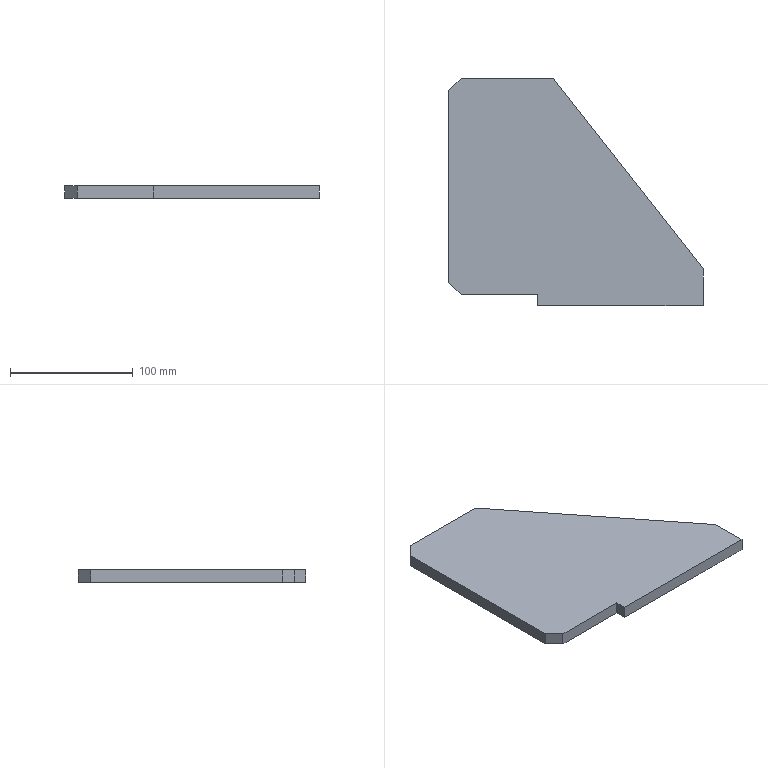Part | STEP file | E3-顶部Beam筋Plate 2 | 1 solid | 11 faces | box 207 x 185 x 10 mm | volume 280920 mm3 | plane 11
STEP:
#1=CARTESIAN_POINT('',(0.,0.,0.));
#2=DIRECTION('',(0.,0.,1.));
#3=DIRECTION('',(1.,0.,0.));
#4=AXIS2_PLACEMENT_3D('',#1,#2,#3);
#5=CARTESIAN_POINT('',(207.,21.,5.));
#6=VERTEX_POINT('',#5);
#7=CARTESIAN_POINT('',(207.,-9.,5.));
#8=VERTEX_POINT('',#7);
#9=CARTESIAN_POINT('',(207.,0.,5.));
#10=DIRECTION('',(0.,-1.,0.));
#11=VECTOR('',#10,1.);
#12=LINE('',#9,#11);
#13=CARTESIAN_POINT('',(207.,0.,-5.));
#14=DIRECTION('',(1.,0.,0.));
#15=DIRECTION('',(0.,0.,1.));
#16=AXIS2_PLACEMENT_3D('',#13,#14,#15);
#17=PLANE('',#16);
#18=CARTESIAN_POINT('',(10.,0.));
#19=DIRECTION('',(0.,1.));
#20=VECTOR('',#19,1.);
#21=LINE('',#18,#20);
#22=(GEOMETRIC_REPRESENTATION_CONTEXT(2)PARAMETRIC_REPRESENTATION_CONTEXT()REPRESENTATION_CONTEXT('',''));
#23=DEFINITIONAL_REPRESENTATION('',(#21),#22);
#24=PCURVE('',#17,#23);
#25=CARTESIAN_POINT('',(0.,0.,5.));
#26=DIRECTION('',(0.,0.,-1.));
#27=DIRECTION('',(1.,0.,0.));
#28=AXIS2_PLACEMENT_3D('',#25,#26,#27);
#29=PLANE('',#28);
#30=CARTESIAN_POINT('',(207.,0.));
#31=DIRECTION('',(0.,1.));
#32=VECTOR('',#31,1.);
#33=LINE('',#30,#32);
#34=(GEOMETRIC_REPRESENTATION_CONTEXT(2)PARAMETRIC_REPRESENTATION_CONTEXT()REPRESENTATION_CONTEXT('',''));
#35=DEFINITIONAL_REPRESENTATION('',(#33),#34);
#36=PCURVE('',#29,#35);
#37=SURFACE_CURVE('',#12,(#24,#36),.PCURVE_S1.);
#38=EDGE_CURVE('',#6,#8,#37,.T.);
#39=ORIENTED_EDGE('',*,*,#38,.T.);
#40=CARTESIAN_POINT('',(207.,-9.,-5.));
#41=VERTEX_POINT('',#40);
#42=CARTESIAN_POINT('',(207.,-9.,-5.));
#43=DIRECTION('',(0.,0.,1.));
#44=VECTOR('',#43,1.);
#45=LINE('',#42,#44);
#46=CARTESIAN_POINT('',(0.,9.));
#47=DIRECTION('',(1.,0.));
#48=VECTOR('',#47,1.);
#49=LINE('',#46,#48);
#50=(GEOMETRIC_REPRESENTATION_CONTEXT(2)PARAMETRIC_REPRESENTATION_CONTEXT()REPRESENTATION_CONTEXT('',''));
#51=DEFINITIONAL_REPRESENTATION('',(#49),#50);
#52=PCURVE('',#17,#51);
#53=CARTESIAN_POINT('',(0.,-9.,-5.));
#54=DIRECTION('',(0.,1.,0.));
#55=DIRECTION('',(-1.,0.,0.));
#56=AXIS2_PLACEMENT_3D('',#53,#54,#55);
#57=PLANE('',#56);
#58=CARTESIAN_POINT('',(-207.,0.));
#59=DIRECTION('',(0.,1.));
#60=VECTOR('',#59,1.);
#61=LINE('',#58,#60);
#62=(GEOMETRIC_REPRESENTATION_CONTEXT(2)PARAMETRIC_REPRESENTATION_CONTEXT()REPRESENTATION_CONTEXT('',''));
#63=DEFINITIONAL_REPRESENTATION('',(#61),#62);
#64=PCURVE('',#57,#63);
#65=SURFACE_CURVE('',#45,(#52,#64),.PCURVE_S1.);
#66=EDGE_CURVE('',#41,#8,#65,.T.);
#67=ORIENTED_EDGE('',*,*,#66,.F.);
#68=CARTESIAN_POINT('',(207.,21.,-5.));
#69=VERTEX_POINT('',#68);
#70=CARTESIAN_POINT('',(207.,0.,-5.));
#71=DIRECTION('',(0.,-1.,0.));
#72=VECTOR('',#71,1.);
#73=LINE('',#70,#72);
#74=CARTESIAN_POINT('',(0.,0.));
#75=DIRECTION('',(0.,1.));
#76=VECTOR('',#75,1.);
#77=LINE('',#74,#76);
#78=(GEOMETRIC_REPRESENTATION_CONTEXT(2)PARAMETRIC_REPRESENTATION_CONTEXT()REPRESENTATION_CONTEXT('',''));
#79=DEFINITIONAL_REPRESENTATION('',(#77),#78);
#80=PCURVE('',#17,#79);
#81=CARTESIAN_POINT('',(0.,0.,-5.));
#82=DIRECTION('',(0.,0.,-1.));
#83=DIRECTION('',(1.,0.,0.));
#84=AXIS2_PLACEMENT_3D('',#81,#82,#83);
#85=PLANE('',#84);
#86=CARTESIAN_POINT('',(207.,0.));
#87=DIRECTION('',(0.,1.));
#88=VECTOR('',#87,1.);
#89=LINE('',#86,#88);
#90=(GEOMETRIC_REPRESENTATION_CONTEXT(2)PARAMETRIC_REPRESENTATION_CONTEXT()REPRESENTATION_CONTEXT('',''));
#91=DEFINITIONAL_REPRESENTATION('',(#89),#90);
#92=PCURVE('',#85,#91);
#93=SURFACE_CURVE('',#73,(#80,#92),.PCURVE_S1.);
#94=EDGE_CURVE('',#69,#41,#93,.T.);
#95=ORIENTED_EDGE('',*,*,#94,.F.);
#96=CARTESIAN_POINT('',(207.,21.,-5.));
#97=DIRECTION('',(0.,0.,1.));
#98=VECTOR('',#97,1.);
#99=LINE('',#96,#98);
#100=CARTESIAN_POINT('',(0.,-21.));
#101=DIRECTION('',(1.,0.));
#102=VECTOR('',#101,1.);
#103=LINE('',#100,#102);
#104=(GEOMETRIC_REPRESENTATION_CONTEXT(2)PARAMETRIC_REPRESENTATION_CONTEXT()REPRESENTATION_CONTEXT('',''));
#105=DEFINITIONAL_REPRESENTATION('',(#103),#104);
#106=PCURVE('',#17,#105);
#107=CARTESIAN_POINT('',(138.022,108.636,-5.));
#108=DIRECTION('',(0.7858,0.6185,0.));
#109=DIRECTION('',(-0.6185,0.7858,0.));
#110=AXIS2_PLACEMENT_3D('',#107,#108,#109);
#111=PLANE('',#110);
#112=CARTESIAN_POINT('',(-111.526,0.));
#113=DIRECTION('',(0.,1.));
#114=VECTOR('',#113,1.);
#115=LINE('',#112,#114);
#116=(GEOMETRIC_REPRESENTATION_CONTEXT(2)PARAMETRIC_REPRESENTATION_CONTEXT()REPRESENTATION_CONTEXT('',''));
#117=DEFINITIONAL_REPRESENTATION('',(#115),#116);
#118=PCURVE('',#111,#117);
#119=SURFACE_CURVE('',#99,(#106,#118),.PCURVE_S1.);
#120=EDGE_CURVE('',#69,#6,#119,.T.);
#121=ORIENTED_EDGE('',*,*,#120,.T.);
#122=EDGE_LOOP('',(#39,#67,#95,#121));
#123=FACE_BOUND('',#122,.T.);
#124=ADVANCED_FACE('',(#123),#17,.T.);
#125=CARTESIAN_POINT('',(85.,176.,5.));
#126=VERTEX_POINT('',#125);
#127=CARTESIAN_POINT('',(138.022,108.636,5.));
#128=DIRECTION('',(0.6185,-0.7858,0.));
#129=VECTOR('',#128,1.);
#130=LINE('',#127,#129);
#131=CARTESIAN_POINT('',(0.,10.));
#132=DIRECTION('',(-1.,0.));
#133=VECTOR('',#132,1.);
#134=LINE('',#131,#133);
#135=(GEOMETRIC_REPRESENTATION_CONTEXT(2)PARAMETRIC_REPRESENTATION_CONTEXT()REPRESENTATION_CONTEXT('',''));
#136=DEFINITIONAL_REPRESENTATION('',(#134),#135);
#137=PCURVE('',#111,#136);
#138=CARTESIAN_POINT('',(138.022,-108.636));
#139=DIRECTION('',(0.6185,0.7858));
#140=VECTOR('',#139,1.);
#141=LINE('',#138,#140);
#142=(GEOMETRIC_REPRESENTATION_CONTEXT(2)PARAMETRIC_REPRESENTATION_CONTEXT()REPRESENTATION_CONTEXT('',''));
#143=DEFINITIONAL_REPRESENTATION('',(#141),#142);
#144=PCURVE('',#29,#143);
#145=SURFACE_CURVE('',#130,(#137,#144),.PCURVE_S1.);
#146=EDGE_CURVE('',#126,#6,#145,.T.);
#147=ORIENTED_EDGE('',*,*,#146,.T.);
#148=ORIENTED_EDGE('',*,*,#120,.F.);
#149=CARTESIAN_POINT('',(85.,176.,-5.));
#150=VERTEX_POINT('',#149);
#151=CARTESIAN_POINT('',(138.022,108.636,-5.));
#152=DIRECTION('',(0.6185,-0.7858,0.));
#153=VECTOR('',#152,1.);
#154=LINE('',#151,#153);
#155=CARTESIAN_POINT('',(0.,0.));
#156=DIRECTION('',(-1.,0.));
#157=VECTOR('',#156,1.);
#158=LINE('',#155,#157);
#159=(GEOMETRIC_REPRESENTATION_CONTEXT(2)PARAMETRIC_REPRESENTATION_CONTEXT()REPRESENTATION_CONTEXT('',''));
#160=DEFINITIONAL_REPRESENTATION('',(#158),#159);
#161=PCURVE('',#111,#160);
#162=CARTESIAN_POINT('',(138.022,-108.636));
#163=DIRECTION('',(0.6185,0.7858));
#164=VECTOR('',#163,1.);
#165=LINE('',#162,#164);
#166=(GEOMETRIC_REPRESENTATION_CONTEXT(2)PARAMETRIC_REPRESENTATION_CONTEXT()REPRESENTATION_CONTEXT('',''));
#167=DEFINITIONAL_REPRESENTATION('',(#165),#166);
#168=PCURVE('',#85,#167);
#169=SURFACE_CURVE('',#154,(#161,#168),.PCURVE_S1.);
#170=EDGE_CURVE('',#150,#69,#169,.T.);
#171=ORIENTED_EDGE('',*,*,#170,.F.);
#172=CARTESIAN_POINT('',(85.,176.,-5.));
#173=DIRECTION('',(0.,0.,1.));
#174=VECTOR('',#173,1.);
#175=LINE('',#172,#174);
#176=CARTESIAN_POINT('',(85.727,0.));
#177=DIRECTION('',(0.,1.));
#178=VECTOR('',#177,1.);
#179=LINE('',#176,#178);
#180=(GEOMETRIC_REPRESENTATION_CONTEXT(2)PARAMETRIC_REPRESENTATION_CONTEXT()REPRESENTATION_CONTEXT('',''));
#181=DEFINITIONAL_REPRESENTATION('',(#179),#180);
#182=PCURVE('',#111,#181);
#183=CARTESIAN_POINT('',(0.,176.,-5.));
#184=DIRECTION('',(0.,1.,0.));
#185=DIRECTION('',(0.,0.,-1.));
#186=AXIS2_PLACEMENT_3D('',#183,#184,#185);
#187=PLANE('',#186);
#188=CARTESIAN_POINT('',(0.,-85.));
#189=DIRECTION('',(-1.,0.));
#190=VECTOR('',#189,1.);
#191=LINE('',#188,#190);
#192=(GEOMETRIC_REPRESENTATION_CONTEXT(2)PARAMETRIC_REPRESENTATION_CONTEXT()REPRESENTATION_CONTEXT('',''));
#193=DEFINITIONAL_REPRESENTATION('',(#191),#192);
#194=PCURVE('',#187,#193);
#195=SURFACE_CURVE('',#175,(#182,#194),.PCURVE_S1.);
#196=EDGE_CURVE('',#150,#126,#195,.T.);
#197=ORIENTED_EDGE('',*,*,#196,.T.);
#198=EDGE_LOOP('',(#147,#148,#171,#197));
#199=FACE_BOUND('',#198,.T.);
#200=ADVANCED_FACE('',(#199),#111,.T.);
#201=CARTESIAN_POINT('',(10.,176.,5.));
#202=VERTEX_POINT('',#201);
#203=CARTESIAN_POINT('',(0.,176.,5.));
#204=DIRECTION('',(1.,0.,0.));
#205=VECTOR('',#204,1.);
#206=LINE('',#203,#205);
#207=CARTESIAN_POINT('',(-10.,0.));
#208=DIRECTION('',(0.,-1.));
#209=VECTOR('',#208,1.);
#210=LINE('',#207,#209);
#211=(GEOMETRIC_REPRESENTATION_CONTEXT(2)PARAMETRIC_REPRESENTATION_CONTEXT()REPRESENTATION_CONTEXT('',''));
#212=DEFINITIONAL_REPRESENTATION('',(#210),#211);
#213=PCURVE('',#187,#212);
#214=CARTESIAN_POINT('',(0.,-176.));
#215=DIRECTION('',(1.,0.));
#216=VECTOR('',#215,1.);
#217=LINE('',#214,#216);
#218=(GEOMETRIC_REPRESENTATION_CONTEXT(2)PARAMETRIC_REPRESENTATION_CONTEXT()REPRESENTATION_CONTEXT('',''));
#219=DEFINITIONAL_REPRESENTATION('',(#217),#218);
#220=PCURVE('',#29,#219);
#221=SURFACE_CURVE('',#206,(#213,#220),.PCURVE_S1.);
#222=EDGE_CURVE('',#202,#126,#221,.T.);
#223=ORIENTED_EDGE('',*,*,#222,.T.);
#224=ORIENTED_EDGE('',*,*,#196,.F.);
#225=CARTESIAN_POINT('',(10.,176.,-5.));
#226=VERTEX_POINT('',#225);
#227=CARTESIAN_POINT('',(0.,176.,-5.));
#228=DIRECTION('',(1.,0.,0.));
#229=VECTOR('',#228,1.);
#230=LINE('',#227,#229);
#231=CARTESIAN_POINT('',(0.,0.));
#232=DIRECTION('',(0.,-1.));
#233=VECTOR('',#232,1.);
#234=LINE('',#231,#233);
#235=(GEOMETRIC_REPRESENTATION_CONTEXT(2)PARAMETRIC_REPRESENTATION_CONTEXT()REPRESENTATION_CONTEXT('',''));
#236=DEFINITIONAL_REPRESENTATION('',(#234),#235);
#237=PCURVE('',#187,#236);
#238=CARTESIAN_POINT('',(0.,-176.));
#239=DIRECTION('',(1.,0.));
#240=VECTOR('',#239,1.);
#241=LINE('',#238,#240);
#242=(GEOMETRIC_REPRESENTATION_CONTEXT(2)PARAMETRIC_REPRESENTATION_CONTEXT()REPRESENTATION_CONTEXT('',''));
#243=DEFINITIONAL_REPRESENTATION('',(#241),#242);
#244=PCURVE('',#85,#243);
#245=SURFACE_CURVE('',#230,(#237,#244),.PCURVE_S1.);
#246=EDGE_CURVE('',#226,#150,#245,.T.);
#247=ORIENTED_EDGE('',*,*,#246,.F.);
#248=CARTESIAN_POINT('',(10.,176.,-5.));
#249=DIRECTION('',(0.,0.,-1.));
#250=VECTOR('',#249,1.);
#251=LINE('',#248,#250);
#252=CARTESIAN_POINT('',(0.,-10.));
#253=DIRECTION('',(1.,0.));
#254=VECTOR('',#253,1.);
#255=LINE('',#252,#254);
#256=(GEOMETRIC_REPRESENTATION_CONTEXT(2)PARAMETRIC_REPRESENTATION_CONTEXT()REPRESENTATION_CONTEXT('',''));
#257=DEFINITIONAL_REPRESENTATION('',(#255),#256);
#258=PCURVE('',#187,#257);
#259=CARTESIAN_POINT('',(0.,166.,-5.));
#260=DIRECTION('',(0.7071,-0.7071,0.));
#261=DIRECTION('',(0.,0.,1.));
#262=AXIS2_PLACEMENT_3D('',#259,#260,#261);
#263=PLANE('',#262);
#264=CARTESIAN_POINT('',(0.,-14.142));
#265=DIRECTION('',(-1.,0.));
#266=VECTOR('',#265,1.);
#267=LINE('',#264,#266);
#268=(GEOMETRIC_REPRESENTATION_CONTEXT(2)PARAMETRIC_REPRESENTATION_CONTEXT()REPRESENTATION_CONTEXT('',''));
#269=DEFINITIONAL_REPRESENTATION('',(#267),#268);
#270=PCURVE('',#263,#269);
#271=SURFACE_CURVE('',#251,(#258,#270),.PCURVE_S1.);
#272=EDGE_CURVE('',#202,#226,#271,.T.);
#273=ORIENTED_EDGE('',*,*,#272,.F.);
#274=EDGE_LOOP('',(#223,#224,#247,#273));
#275=FACE_BOUND('',#274,.T.);
#276=ADVANCED_FACE('',(#275),#187,.T.);
#277=CARTESIAN_POINT('',(0.,10.,5.));
#278=VERTEX_POINT('',#277);
#279=CARTESIAN_POINT('',(0.,166.,5.));
#280=VERTEX_POINT('',#279);
#281=CARTESIAN_POINT('',(0.,0.,5.));
#282=DIRECTION('',(0.,1.,0.));
#283=VECTOR('',#282,1.);
#284=LINE('',#281,#283);
#285=CARTESIAN_POINT('',(0.,0.,-5.));
#286=DIRECTION('',(-1.,0.,0.));
#287=DIRECTION('',(0.,0.,-1.));
#288=AXIS2_PLACEMENT_3D('',#285,#286,#287);
#289=PLANE('',#288);
#290=CARTESIAN_POINT('',(-10.,0.));
#291=DIRECTION('',(0.,-1.));
#292=VECTOR('',#291,1.);
#293=LINE('',#290,#292);
#294=(GEOMETRIC_REPRESENTATION_CONTEXT(2)PARAMETRIC_REPRESENTATION_CONTEXT()REPRESENTATION_CONTEXT('',''));
#295=DEFINITIONAL_REPRESENTATION('',(#293),#294);
#296=PCURVE('',#289,#295);
#297=CARTESIAN_POINT('',(0.,0.));
#298=DIRECTION('',(0.,-1.));
#299=VECTOR('',#298,1.);
#300=LINE('',#297,#299);
#301=(GEOMETRIC_REPRESENTATION_CONTEXT(2)PARAMETRIC_REPRESENTATION_CONTEXT()REPRESENTATION_CONTEXT('',''));
#302=DEFINITIONAL_REPRESENTATION('',(#300),#301);
#303=PCURVE('',#29,#302);
#304=SURFACE_CURVE('',#284,(#296,#303),.PCURVE_S1.);
#305=EDGE_CURVE('',#278,#280,#304,.T.);
#306=ORIENTED_EDGE('',*,*,#305,.T.);
#307=CARTESIAN_POINT('',(0.,166.,-5.));
#308=VERTEX_POINT('',#307);
#309=CARTESIAN_POINT('',(0.,166.,-5.));
#310=DIRECTION('',(0.,0.,1.));
#311=VECTOR('',#310,1.);
#312=LINE('',#309,#311);
#313=CARTESIAN_POINT('',(0.,-166.));
#314=DIRECTION('',(-1.,0.));
#315=VECTOR('',#314,1.);
#316=LINE('',#313,#315);
#317=(GEOMETRIC_REPRESENTATION_CONTEXT(2)PARAMETRIC_REPRESENTATION_CONTEXT()REPRESENTATION_CONTEXT('',''));
#318=DEFINITIONAL_REPRESENTATION('',(#316),#317);
#319=PCURVE('',#289,#318);
#320=CARTESIAN_POINT('',(0.,0.));
#321=DIRECTION('',(1.,0.));
#322=VECTOR('',#321,1.);
#323=LINE('',#320,#322);
#324=(GEOMETRIC_REPRESENTATION_CONTEXT(2)PARAMETRIC_REPRESENTATION_CONTEXT()REPRESENTATION_CONTEXT('',''));
#325=DEFINITIONAL_REPRESENTATION('',(#323),#324);
#326=PCURVE('',#263,#325);
#327=SURFACE_CURVE('',#312,(#319,#326),.PCURVE_S1.);
#328=EDGE_CURVE('',#308,#280,#327,.T.);
#329=ORIENTED_EDGE('',*,*,#328,.F.);
#330=CARTESIAN_POINT('',(0.,10.,-5.));
#331=VERTEX_POINT('',#330);
#332=CARTESIAN_POINT('',(0.,0.,-5.));
#333=DIRECTION('',(0.,1.,0.));
#334=VECTOR('',#333,1.);
#335=LINE('',#332,#334);
#336=CARTESIAN_POINT('',(0.,0.));
#337=DIRECTION('',(0.,-1.));
#338=VECTOR('',#337,1.);
#339=LINE('',#336,#338);
#340=(GEOMETRIC_REPRESENTATION_CONTEXT(2)PARAMETRIC_REPRESENTATION_CONTEXT()REPRESENTATION_CONTEXT('',''));
#341=DEFINITIONAL_REPRESENTATION('',(#339),#340);
#342=PCURVE('',#289,#341);
#343=CARTESIAN_POINT('',(0.,0.));
#344=DIRECTION('',(0.,-1.));
#345=VECTOR('',#344,1.);
#346=LINE('',#343,#345);
#347=(GEOMETRIC_REPRESENTATION_CONTEXT(2)PARAMETRIC_REPRESENTATION_CONTEXT()REPRESENTATION_CONTEXT('',''));
#348=DEFINITIONAL_REPRESENTATION('',(#346),#347);
#349=PCURVE('',#85,#348);
#350=SURFACE_CURVE('',#335,(#342,#349),.PCURVE_S1.);
#351=EDGE_CURVE('',#331,#308,#350,.T.);
#352=ORIENTED_EDGE('',*,*,#351,.F.);
#353=CARTESIAN_POINT('',(0.,10.,-5.));
#354=DIRECTION('',(0.,0.,-1.));
#355=VECTOR('',#354,1.);
#356=LINE('',#353,#355);
#357=CARTESIAN_POINT('',(0.,-10.));
#358=DIRECTION('',(1.,0.));
#359=VECTOR('',#358,1.);
#360=LINE('',#357,#359);
#361=(GEOMETRIC_REPRESENTATION_CONTEXT(2)PARAMETRIC_REPRESENTATION_CONTEXT()REPRESENTATION_CONTEXT('',''));
#362=DEFINITIONAL_REPRESENTATION('',(#360),#361);
#363=PCURVE('',#289,#362);
#364=CARTESIAN_POINT('',(10.,0.,-5.));
#365=DIRECTION('',(-0.7071,-0.7071,0.));
#366=DIRECTION('',(0.,0.,-1.));
#367=AXIS2_PLACEMENT_3D('',#364,#365,#366);
#368=PLANE('',#367);
#369=CARTESIAN_POINT('',(0.,-14.142));
#370=DIRECTION('',(1.,0.));
#371=VECTOR('',#370,1.);
#372=LINE('',#369,#371);
#373=(GEOMETRIC_REPRESENTATION_CONTEXT(2)PARAMETRIC_REPRESENTATION_CONTEXT()REPRESENTATION_CONTEXT('',''));
#374=DEFINITIONAL_REPRESENTATION('',(#372),#373);
#375=PCURVE('',#368,#374);
#376=SURFACE_CURVE('',#356,(#363,#375),.PCURVE_S1.);
#377=EDGE_CURVE('',#278,#331,#376,.T.);
#378=ORIENTED_EDGE('',*,*,#377,.F.);
#379=EDGE_LOOP('',(#306,#329,#352,#378));
#380=FACE_BOUND('',#379,.T.);
#381=ADVANCED_FACE('',(#380),#289,.T.);
#382=CARTESIAN_POINT('',(10.,0.,-5.));
#383=VERTEX_POINT('',#382);
#384=CARTESIAN_POINT('',(72.,0.,-5.));
#385=VERTEX_POINT('',#384);
#386=CARTESIAN_POINT('',(0.,0.,-5.));
#387=DIRECTION('',(1.,0.,0.));
#388=VECTOR('',#387,1.);
#389=LINE('',#386,#388);
#390=CARTESIAN_POINT('',(0.,0.,-5.));
#391=DIRECTION('',(0.,1.,0.));
#392=DIRECTION('',(0.,0.,-1.));
#393=AXIS2_PLACEMENT_3D('',#390,#391,#392);
#394=PLANE('',#393);
#395=CARTESIAN_POINT('',(0.,0.));
#396=DIRECTION('',(0.,-1.));
#397=VECTOR('',#396,1.);
#398=LINE('',#395,#397);
#399=(GEOMETRIC_REPRESENTATION_CONTEXT(2)PARAMETRIC_REPRESENTATION_CONTEXT()REPRESENTATION_CONTEXT('',''));
#400=DEFINITIONAL_REPRESENTATION('',(#398),#399);
#401=PCURVE('',#394,#400);
#402=CARTESIAN_POINT('',(0.,0.));
#403=DIRECTION('',(1.,0.));
#404=VECTOR('',#403,1.);
#405=LINE('',#402,#404);
#406=(GEOMETRIC_REPRESENTATION_CONTEXT(2)PARAMETRIC_REPRESENTATION_CONTEXT()REPRESENTATION_CONTEXT('',''));
#407=DEFINITIONAL_REPRESENTATION('',(#405),#406);
#408=PCURVE('',#85,#407);
#409=SURFACE_CURVE('',#389,(#401,#408),.PCURVE_S1.);
#410=EDGE_CURVE('',#383,#385,#409,.T.);
#411=ORIENTED_EDGE('',*,*,#410,.T.);
#412=CARTESIAN_POINT('',(72.,0.,5.));
#413=VERTEX_POINT('',#412);
#414=CARTESIAN_POINT('',(72.,0.,-5.));
#415=DIRECTION('',(0.,0.,1.));
#416=VECTOR('',#415,1.);
#417=LINE('',#414,#416);
#418=CARTESIAN_POINT('',(0.,-72.));
#419=DIRECTION('',(-1.,0.));
#420=VECTOR('',#419,1.);
#421=LINE('',#418,#420);
#422=(GEOMETRIC_REPRESENTATION_CONTEXT(2)PARAMETRIC_REPRESENTATION_CONTEXT()REPRESENTATION_CONTEXT('',''));
#423=DEFINITIONAL_REPRESENTATION('',(#421),#422);
#424=PCURVE('',#394,#423);
#425=CARTESIAN_POINT('',(72.,0.,-5.));
#426=DIRECTION('',(1.,0.,0.));
#427=DIRECTION('',(0.,0.,1.));
#428=AXIS2_PLACEMENT_3D('',#425,#426,#427);
#429=PLANE('',#428);
#430=CARTESIAN_POINT('',(0.,0.));
#431=DIRECTION('',(1.,0.));
#432=VECTOR('',#431,1.);
#433=LINE('',#430,#432);
#434=(GEOMETRIC_REPRESENTATION_CONTEXT(2)PARAMETRIC_REPRESENTATION_CONTEXT()REPRESENTATION_CONTEXT('',''));
#435=DEFINITIONAL_REPRESENTATION('',(#433),#434);
#436=PCURVE('',#429,#435);
#437=SURFACE_CURVE('',#417,(#424,#436),.PCURVE_S1.);
#438=EDGE_CURVE('',#385,#413,#437,.T.);
#439=ORIENTED_EDGE('',*,*,#438,.T.);
#440=CARTESIAN_POINT('',(10.,0.,5.));
#441=VERTEX_POINT('',#440);
#442=CARTESIAN_POINT('',(0.,0.,5.));
#443=DIRECTION('',(1.,0.,0.));
#444=VECTOR('',#443,1.);
#445=LINE('',#442,#444);
#446=CARTESIAN_POINT('',(-10.,0.));
#447=DIRECTION('',(0.,-1.));
#448=VECTOR('',#447,1.);
#449=LINE('',#446,#448);
#450=(GEOMETRIC_REPRESENTATION_CONTEXT(2)PARAMETRIC_REPRESENTATION_CONTEXT()REPRESENTATION_CONTEXT('',''));
#451=DEFINITIONAL_REPRESENTATION('',(#449),#450);
#452=PCURVE('',#394,#451);
#453=CARTESIAN_POINT('',(0.,0.));
#454=DIRECTION('',(1.,0.));
#455=VECTOR('',#454,1.);
#456=LINE('',#453,#455);
#457=(GEOMETRIC_REPRESENTATION_CONTEXT(2)PARAMETRIC_REPRESENTATION_CONTEXT()REPRESENTATION_CONTEXT('',''));
#458=DEFINITIONAL_REPRESENTATION('',(#456),#457);
#459=PCURVE('',#29,#458);
#460=SURFACE_CURVE('',#445,(#452,#459),.PCURVE_S1.);
#461=EDGE_CURVE('',#441,#413,#460,.T.);
#462=ORIENTED_EDGE('',*,*,#461,.F.);
#463=CARTESIAN_POINT('',(10.,0.,5.));
#464=DIRECTION('',(0.,0.,1.));
#465=VECTOR('',#464,1.);
#466=LINE('',#463,#465);
#467=CARTESIAN_POINT('',(-10.,-10.));
#468=DIRECTION('',(-1.,0.));
#469=VECTOR('',#468,1.);
#470=LINE('',#467,#469);
#471=(GEOMETRIC_REPRESENTATION_CONTEXT(2)PARAMETRIC_REPRESENTATION_CONTEXT()REPRESENTATION_CONTEXT('',''));
#472=DEFINITIONAL_REPRESENTATION('',(#470),#471);
#473=PCURVE('',#394,#472);
#474=CARTESIAN_POINT('',(-10.,0.));
#475=DIRECTION('',(-1.,0.));
#476=VECTOR('',#475,1.);
#477=LINE('',#474,#476);
#478=(GEOMETRIC_REPRESENTATION_CONTEXT(2)PARAMETRIC_REPRESENTATION_CONTEXT()REPRESENTATION_CONTEXT('',''));
#479=DEFINITIONAL_REPRESENTATION('',(#477),#478);
#480=PCURVE('',#368,#479);
#481=SURFACE_CURVE('',#466,(#473,#480),.PCURVE_S1.);
#482=EDGE_CURVE('',#383,#441,#481,.T.);
#483=ORIENTED_EDGE('',*,*,#482,.F.);
#484=EDGE_LOOP('',(#411,#439,#462,#483));
#485=FACE_BOUND('',#484,.T.);
#486=ADVANCED_FACE('',(#485),#394,.F.);
#487=CARTESIAN_POINT('',(72.,-9.,5.));
#488=VERTEX_POINT('',#487);
#489=CARTESIAN_POINT('',(72.,0.,5.));
#490=DIRECTION('',(0.,-1.,0.));
#491=VECTOR('',#490,1.);
#492=LINE('',#489,#491);
#493=CARTESIAN_POINT('',(10.,0.));
#494=DIRECTION('',(0.,1.));
#495=VECTOR('',#494,1.);
#496=LINE('',#493,#495);
#497=(GEOMETRIC_REPRESENTATION_CONTEXT(2)PARAMETRIC_REPRESENTATION_CONTEXT()REPRESENTATION_CONTEXT('',''));
#498=DEFINITIONAL_REPRESENTATION('',(#496),#497);
#499=PCURVE('',#429,#498);
#500=CARTESIAN_POINT('',(72.,0.));
#501=DIRECTION('',(0.,1.));
#502=VECTOR('',#501,1.);
#503=LINE('',#500,#502);
#504=(GEOMETRIC_REPRESENTATION_CONTEXT(2)PARAMETRIC_REPRESENTATION_CONTEXT()REPRESENTATION_CONTEXT('',''));
#505=DEFINITIONAL_REPRESENTATION('',(#503),#504);
#506=PCURVE('',#29,#505);
#507=SURFACE_CURVE('',#492,(#499,#506),.PCURVE_S1.);
#508=EDGE_CURVE('',#413,#488,#507,.T.);
#509=ORIENTED_EDGE('',*,*,#508,.F.);
#510=ORIENTED_EDGE('',*,*,#438,.F.);
#511=CARTESIAN_POINT('',(72.,-9.,-5.));
#512=VERTEX_POINT('',#511);
#513=CARTESIAN_POINT('',(72.,0.,-5.));
#514=DIRECTION('',(0.,-1.,0.));
#515=VECTOR('',#514,1.);
#516=LINE('',#513,#515);
#517=CARTESIAN_POINT('',(0.,0.));
#518=DIRECTION('',(0.,1.));
#519=VECTOR('',#518,1.);
#520=LINE('',#517,#519);
#521=(GEOMETRIC_REPRESENTATION_CONTEXT(2)PARAMETRIC_REPRESENTATION_CONTEXT()REPRESENTATION_CONTEXT('',''));
#522=DEFINITIONAL_REPRESENTATION('',(#520),#521);
#523=PCURVE('',#429,#522);
#524=CARTESIAN_POINT('',(72.,0.));
#525=DIRECTION('',(0.,1.));
#526=VECTOR('',#525,1.);
#527=LINE('',#524,#526);
#528=(GEOMETRIC_REPRESENTATION_CONTEXT(2)PARAMETRIC_REPRESENTATION_CONTEXT()REPRESENTATION_CONTEXT('',''));
#529=DEFINITIONAL_REPRESENTATION('',(#527),#528);
#530=PCURVE('',#85,#529);
#531=SURFACE_CURVE('',#516,(#523,#530),.PCURVE_S1.);
#532=EDGE_CURVE('',#385,#512,#531,.T.);
#533=ORIENTED_EDGE('',*,*,#532,.T.);
#534=CARTESIAN_POINT('',(72.,-9.,-5.));
#535=DIRECTION('',(0.,0.,1.));
#536=VECTOR('',#535,1.);
#537=LINE('',#534,#536);
#538=CARTESIAN_POINT('',(0.,9.));
#539=DIRECTION('',(1.,0.));
#540=VECTOR('',#539,1.);
#541=LINE('',#538,#540);
#542=(GEOMETRIC_REPRESENTATION_CONTEXT(2)PARAMETRIC_REPRESENTATION_CONTEXT()REPRESENTATION_CONTEXT('',''));
#543=DEFINITIONAL_REPRESENTATION('',(#541),#542);
#544=PCURVE('',#429,#543);
#545=CARTESIAN_POINT('',(-72.,0.));
#546=DIRECTION('',(0.,1.));
#547=VECTOR('',#546,1.);
#548=LINE('',#545,#547);
#549=(GEOMETRIC_REPRESENTATION_CONTEXT(2)PARAMETRIC_REPRESENTATION_CONTEXT()REPRESENTATION_CONTEXT('',''));
#550=DEFINITIONAL_REPRESENTATION('',(#548),#549);
#551=PCURVE('',#57,#550);
#552=SURFACE_CURVE('',#537,(#544,#551),.PCURVE_S1.);
#553=EDGE_CURVE('',#512,#488,#552,.T.);
#554=ORIENTED_EDGE('',*,*,#553,.T.);
#555=EDGE_LOOP('',(#509,#510,#533,#554));
#556=FACE_BOUND('',#555,.T.);
#557=ADVANCED_FACE('',(#556),#429,.F.);
#558=CARTESIAN_POINT('',(0.,-9.,5.));
#559=DIRECTION('',(1.,0.,0.));
#560=VECTOR('',#559,1.);
#561=LINE('',#558,#560);
#562=CARTESIAN_POINT('',(0.,10.));
#563=DIRECTION('',(-1.,0.));
#564=VECTOR('',#563,1.);
#565=LINE('',#562,#564);
#566=(GEOMETRIC_REPRESENTATION_CONTEXT(2)PARAMETRIC_REPRESENTATION_CONTEXT()REPRESENTATION_CONTEXT('',''));
#567=DEFINITIONAL_REPRESENTATION('',(#565),#566);
#568=PCURVE('',#57,#567);
#569=CARTESIAN_POINT('',(0.,9.));
#570=DIRECTION('',(1.,0.));
#571=VECTOR('',#570,1.);
#572=LINE('',#569,#571);
#573=(GEOMETRIC_REPRESENTATION_CONTEXT(2)PARAMETRIC_REPRESENTATION_CONTEXT()REPRESENTATION_CONTEXT('',''));
#574=DEFINITIONAL_REPRESENTATION('',(#572),#573);
#575=PCURVE('',#29,#574);
#576=SURFACE_CURVE('',#561,(#568,#575),.PCURVE_S1.);
#577=EDGE_CURVE('',#488,#8,#576,.T.);
#578=ORIENTED_EDGE('',*,*,#577,.F.);
#579=ORIENTED_EDGE('',*,*,#553,.F.);
#580=CARTESIAN_POINT('',(0.,-9.,-5.));
#581=DIRECTION('',(1.,0.,0.));
#582=VECTOR('',#581,1.);
#583=LINE('',#580,#582);
#584=CARTESIAN_POINT('',(0.,0.));
#585=DIRECTION('',(-1.,0.));
#586=VECTOR('',#585,1.);
#587=LINE('',#584,#586);
#588=(GEOMETRIC_REPRESENTATION_CONTEXT(2)PARAMETRIC_REPRESENTATION_CONTEXT()REPRESENTATION_CONTEXT('',''));
#589=DEFINITIONAL_REPRESENTATION('',(#587),#588);
#590=PCURVE('',#57,#589);
#591=CARTESIAN_POINT('',(0.,9.));
#592=DIRECTION('',(1.,0.));
#593=VECTOR('',#592,1.);
#594=LINE('',#591,#593);
#595=(GEOMETRIC_REPRESENTATION_CONTEXT(2)PARAMETRIC_REPRESENTATION_CONTEXT()REPRESENTATION_CONTEXT('',''));
#596=DEFINITIONAL_REPRESENTATION('',(#594),#595);
#597=PCURVE('',#85,#596);
#598=SURFACE_CURVE('',#583,(#590,#597),.PCURVE_S1.);
#599=EDGE_CURVE('',#512,#41,#598,.T.);
#600=ORIENTED_EDGE('',*,*,#599,.T.);
#601=ORIENTED_EDGE('',*,*,#66,.T.);
#602=EDGE_LOOP('',(#578,#579,#600,#601));
#603=FACE_BOUND('',#602,.T.);
#604=ADVANCED_FACE('',(#603),#57,.F.);
#605=ORIENTED_EDGE('',*,*,#351,.T.);
#606=CARTESIAN_POINT('',(-83.,83.,-5.));
#607=DIRECTION('',(-0.7071,-0.7071,0.));
#608=VECTOR('',#607,1.);
#609=LINE('',#606,#608);
#610=CARTESIAN_POINT('',(-83.,-83.));
#611=DIRECTION('',(-0.7071,0.7071));
#612=VECTOR('',#611,1.);
#613=LINE('',#610,#612);
#614=(GEOMETRIC_REPRESENTATION_CONTEXT(2)PARAMETRIC_REPRESENTATION_CONTEXT()REPRESENTATION_CONTEXT('',''));
#615=DEFINITIONAL_REPRESENTATION('',(#613),#614);
#616=PCURVE('',#85,#615);
#617=CARTESIAN_POINT('',(0.,117.38));
#618=DIRECTION('',(0.,1.));
#619=VECTOR('',#618,1.);
#620=LINE('',#617,#619);
#621=(GEOMETRIC_REPRESENTATION_CONTEXT(2)PARAMETRIC_REPRESENTATION_CONTEXT()REPRESENTATION_CONTEXT('',''));
#622=DEFINITIONAL_REPRESENTATION('',(#620),#621);
#623=PCURVE('',#263,#622);
#624=SURFACE_CURVE('',#609,(#616,#623),.PCURVE_S1.);
#625=EDGE_CURVE('',#226,#308,#624,.T.);
#626=ORIENTED_EDGE('',*,*,#625,.F.);
#627=ORIENTED_EDGE('',*,*,#246,.T.);
#628=ORIENTED_EDGE('',*,*,#170,.T.);
#629=ORIENTED_EDGE('',*,*,#94,.T.);
#630=ORIENTED_EDGE('',*,*,#599,.F.);
#631=ORIENTED_EDGE('',*,*,#532,.F.);
#632=ORIENTED_EDGE('',*,*,#410,.F.);
#633=CARTESIAN_POINT('',(5.,5.,-5.));
#634=DIRECTION('',(0.7071,-0.7071,0.));
#635=VECTOR('',#634,1.);
#636=LINE('',#633,#635);
#637=CARTESIAN_POINT('',(5.,-5.));
#638=DIRECTION('',(0.7071,0.7071));
#639=VECTOR('',#638,1.);
#640=LINE('',#637,#639);
#641=(GEOMETRIC_REPRESENTATION_CONTEXT(2)PARAMETRIC_REPRESENTATION_CONTEXT()REPRESENTATION_CONTEXT('',''));
#642=DEFINITIONAL_REPRESENTATION('',(#640),#641);
#643=PCURVE('',#85,#642);
#644=CARTESIAN_POINT('',(0.,-7.071));
#645=DIRECTION('',(0.,1.));
#646=VECTOR('',#645,1.);
#647=LINE('',#644,#646);
#648=(GEOMETRIC_REPRESENTATION_CONTEXT(2)PARAMETRIC_REPRESENTATION_CONTEXT()REPRESENTATION_CONTEXT('',''));
#649=DEFINITIONAL_REPRESENTATION('',(#647),#648);
#650=PCURVE('',#368,#649);
#651=SURFACE_CURVE('',#636,(#643,#650),.PCURVE_S1.);
#652=EDGE_CURVE('',#331,#383,#651,.T.);
#653=ORIENTED_EDGE('',*,*,#652,.F.);
#654=EDGE_LOOP('',(#605,#626,#627,#628,#629,#630,#631,#632,#653));
#655=FACE_BOUND('',#654,.T.);
#656=ADVANCED_FACE('',(#655),#85,.T.);
#657=ORIENTED_EDGE('',*,*,#461,.T.);
#658=ORIENTED_EDGE('',*,*,#508,.T.);
#659=ORIENTED_EDGE('',*,*,#577,.T.);
#660=ORIENTED_EDGE('',*,*,#38,.F.);
#661=ORIENTED_EDGE('',*,*,#146,.F.);
#662=ORIENTED_EDGE('',*,*,#222,.F.);
#663=CARTESIAN_POINT('',(0.,166.,5.));
#664=DIRECTION('',(0.7071,0.7071,0.));
#665=VECTOR('',#664,1.);
#666=LINE('',#663,#665);
#667=CARTESIAN_POINT('',(0.,-166.));
#668=DIRECTION('',(0.7071,-0.7071));
#669=VECTOR('',#668,1.);
#670=LINE('',#667,#669);
#671=(GEOMETRIC_REPRESENTATION_CONTEXT(2)PARAMETRIC_REPRESENTATION_CONTEXT()REPRESENTATION_CONTEXT('',''));
#672=DEFINITIONAL_REPRESENTATION('',(#670),#671);
#673=PCURVE('',#29,#672);
#674=CARTESIAN_POINT('',(10.,0.));
#675=DIRECTION('',(0.,-1.));
#676=VECTOR('',#675,1.);
#677=LINE('',#674,#676);
#678=(GEOMETRIC_REPRESENTATION_CONTEXT(2)PARAMETRIC_REPRESENTATION_CONTEXT()REPRESENTATION_CONTEXT('',''));
#679=DEFINITIONAL_REPRESENTATION('',(#677),#678);
#680=PCURVE('',#263,#679);
#681=SURFACE_CURVE('',#666,(#673,#680),.PCURVE_S1.);
#682=EDGE_CURVE('',#280,#202,#681,.T.);
#683=ORIENTED_EDGE('',*,*,#682,.F.);
#684=ORIENTED_EDGE('',*,*,#305,.F.);
#685=CARTESIAN_POINT('',(10.,0.,5.));
#686=DIRECTION('',(-0.7071,0.7071,0.));
#687=VECTOR('',#686,1.);
#688=LINE('',#685,#687);
#689=CARTESIAN_POINT('',(10.,0.));
#690=DIRECTION('',(-0.7071,-0.7071));
#691=VECTOR('',#690,1.);
#692=LINE('',#689,#691);
#693=(GEOMETRIC_REPRESENTATION_CONTEXT(2)PARAMETRIC_REPRESENTATION_CONTEXT()REPRESENTATION_CONTEXT('',''));
#694=DEFINITIONAL_REPRESENTATION('',(#692),#693);
#695=PCURVE('',#29,#694);
#696=CARTESIAN_POINT('',(-10.,0.));
#697=DIRECTION('',(0.,-1.));
#698=VECTOR('',#697,1.);
#699=LINE('',#696,#698);
#700=(GEOMETRIC_REPRESENTATION_CONTEXT(2)PARAMETRIC_REPRESENTATION_CONTEXT()REPRESENTATION_CONTEXT('',''));
#701=DEFINITIONAL_REPRESENTATION('',(#699),#700);
#702=PCURVE('',#368,#701);
#703=SURFACE_CURVE('',#688,(#695,#702),.PCURVE_S1.);
#704=EDGE_CURVE('',#441,#278,#703,.T.);
#705=ORIENTED_EDGE('',*,*,#704,.F.);
#706=EDGE_LOOP('',(#657,#658,#659,#660,#661,#662,#683,#684,#705));
#707=FACE_BOUND('',#706,.T.);
#708=ADVANCED_FACE('',(#707),#29,.F.);
#709=ORIENTED_EDGE('',*,*,#652,.T.);
#710=ORIENTED_EDGE('',*,*,#482,.T.);
#711=ORIENTED_EDGE('',*,*,#704,.T.);
#712=ORIENTED_EDGE('',*,*,#377,.T.);
#713=EDGE_LOOP('',(#709,#710,#711,#712));
#714=FACE_BOUND('',#713,.T.);
#715=ADVANCED_FACE('',(#714),#368,.T.);
#716=ORIENTED_EDGE('',*,*,#625,.T.);
#717=ORIENTED_EDGE('',*,*,#328,.T.);
#718=ORIENTED_EDGE('',*,*,#682,.T.);
#719=ORIENTED_EDGE('',*,*,#272,.T.);
#720=EDGE_LOOP('',(#716,#717,#718,#719));
#721=FACE_BOUND('',#720,.T.);
#722=ADVANCED_FACE('',(#721),#263,.F.);
#723=CLOSED_SHELL('',(#124,#200,#276,#381,#486,#557,#604,#656,#708,#715,#722));
#724=MANIFOLD_SOLID_BREP('',#723);
#725=(LENGTH_UNIT()NAMED_UNIT(*)SI_UNIT(.MILLI.,.METRE.));
#726=UNCERTAINTY_MEASURE_WITH_UNIT(LENGTH_MEASURE(0.0000001),#725,'','');
#727=(NAMED_UNIT(*)PLANE_ANGLE_UNIT()SI_UNIT($,.RADIAN.));
#728=(NAMED_UNIT(*)SI_UNIT($,.STERADIAN.)SOLID_ANGLE_UNIT());
#729=(GEOMETRIC_REPRESENTATION_CONTEXT(3)GLOBAL_UNCERTAINTY_ASSIGNED_CONTEXT((#726))GLOBAL_UNIT_ASSIGNED_CONTEXT((#725,#727,#728))REPRESENTATION_CONTEXT('',''));
#730=ADVANCED_BREP_SHAPE_REPRESENTATION('',(#4,#724),#729);